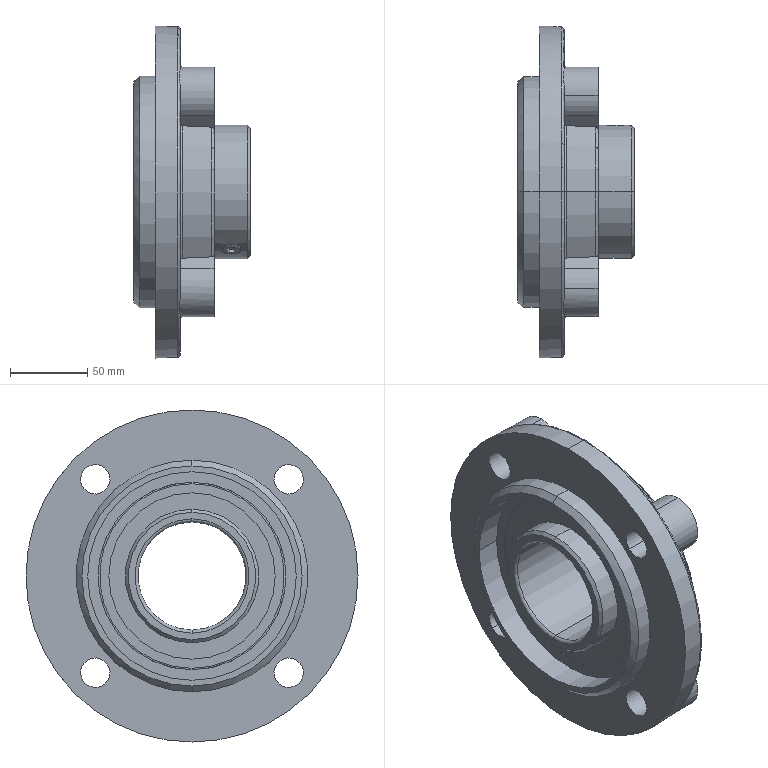Part | SolidWorks | features BaseBody 1 | 1 solid | 154 faces | box 75.4 x 215 x 215 mm | volume 900645 mm3 | cylinder 50 | plane 42 | cone 27 | torus 26 | sphere 9 | commonest cylinder face diameters 1.5 x8 19 x8 86.5 x8 36.4 x6 12 x4 107.713 x4